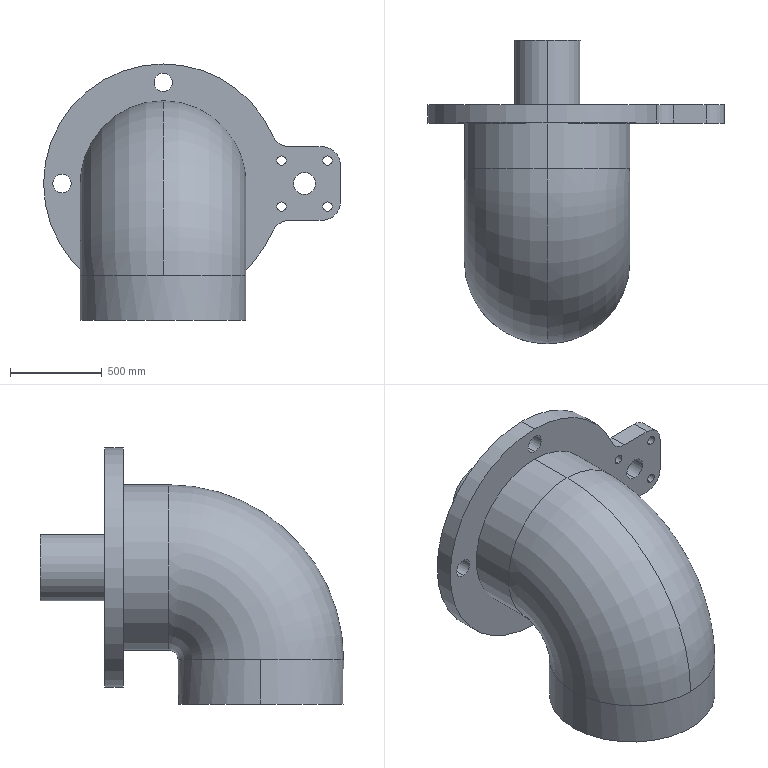Part | SolidWorks | features ICE 9, MoveFace 2, Extrusion 1, Fillet 1, MirrorPattern 1, Sweep 1 | 1 solid | 38 faces | box 1613 x 1648 x 1392 mm | volume 988148338 mm3 | cylinder 29 | plane 7 | torus 2 | commonest cylinder face diameters 50 x8 100 x6 200 x4 900 x4 1300 x3 120 x2
STEP:
#1=CARTESIAN_POINT('',(0.,-298.,-450.));
#2=VERTEX_POINT('',#1);
#3=CARTESIAN_POINT('',(0.,-298.,450.));
#4=VERTEX_POINT('',#3);
#5=CARTESIAN_POINT('',(0.,-298.,0.));
#6=DIRECTION('',(0.,-1.,0.));
#7=DIRECTION('',(0.,0.,-1.));
#8=AXIS2_PLACEMENT_3D('',#5,#6,#7);
#9=CIRCLE('',#8,450.);
#10=EDGE_CURVE('',#2,#4,#9,.T.);
#11=ORIENTED_EDGE('',*,*,#10,.T.);
#12=CARTESIAN_POINT('',(0.,-1248.,-500.));
#13=VERTEX_POINT('',#12);
#14=CARTESIAN_POINT('',(0.,-298.,-500.));
#15=DIRECTION('',(1.,0.,0.));
#16=DIRECTION('',(0.,0.,-1.));
#17=AXIS2_PLACEMENT_3D('',#14,#15,#16);
#18=CIRCLE('',#17,950.);
#19=EDGE_CURVE('',#4,#13,#18,.T.);
#20=ORIENTED_EDGE('',*,*,#19,.T.);
#21=CARTESIAN_POINT('',(450.,-798.,-500.));
#22=VERTEX_POINT('',#21);
#23=CARTESIAN_POINT('',(0.,-798.,-500.));
#24=DIRECTION('',(0.,0.,-1.));
#25=DIRECTION('',(0.,1.,0.));
#26=AXIS2_PLACEMENT_3D('',#23,#24,#25);
#27=CIRCLE('',#26,450.);
#28=EDGE_CURVE('',#22,#13,#27,.T.);
#29=ORIENTED_EDGE('',*,*,#28,.F.);
#30=CARTESIAN_POINT('',(0.,-348.,-500.));
#31=VERTEX_POINT('',#30);
#32=CARTESIAN_POINT('',(0.,-798.,-500.));
#33=DIRECTION('',(0.,0.,-1.));
#34=DIRECTION('',(0.,1.,0.));
#35=AXIS2_PLACEMENT_3D('',#32,#33,#34);
#36=CIRCLE('',#35,450.);
#37=EDGE_CURVE('',#31,#22,#36,.T.);
#38=ORIENTED_EDGE('',*,*,#37,.F.);
#39=CARTESIAN_POINT('',(0.,-298.,-500.));
#40=DIRECTION('',(1.,0.,0.));
#41=DIRECTION('',(0.,0.,-1.));
#42=AXIS2_PLACEMENT_3D('',#39,#40,#41);
#43=CIRCLE('',#42,50.);
#44=EDGE_CURVE('',#2,#31,#43,.T.);
#45=ORIENTED_EDGE('',*,*,#44,.F.);
#46=EDGE_LOOP('',(#11,#20,#29,#38,#45));
#47=FACE_OUTER_BOUND('',#46,.T.);
#48=CARTESIAN_POINT('',(0.,-298.,-500.));
#49=DIRECTION('',(1.,0.,0.));
#50=DIRECTION('',(0.,0.,-1.));
#51=AXIS2_PLACEMENT_3D('',#48,#49,#50);
#52=TOROIDAL_SURFACE('',#51,500.,450.);
#53=ADVANCED_FACE('',(#47),#52,.T.);
#54=CARTESIAN_POINT('',(-450.,-798.,-500.));
#55=VERTEX_POINT('',#54);
#56=CARTESIAN_POINT('',(0.,-798.,-500.));
#57=DIRECTION('',(0.,0.,-1.));
#58=DIRECTION('',(0.,1.,0.));
#59=AXIS2_PLACEMENT_3D('',#56,#57,#58);
#60=CIRCLE('',#59,450.);
#61=EDGE_CURVE('',#55,#31,#60,.T.);
#62=ORIENTED_EDGE('',*,*,#61,.T.);
#63=ORIENTED_EDGE('',*,*,#37,.T.);
#64=CARTESIAN_POINT('',(450.,-798.,-742.));
#65=VERTEX_POINT('',#64);
#66=CARTESIAN_POINT('',(450.,-798.,-500.));
#67=DIRECTION('',(0.,0.,-1.));
#68=VECTOR('',#67,1000.);
#69=LINE('',#66,#68);
#70=EDGE_CURVE('',#22,#65,#69,.T.);
#71=ORIENTED_EDGE('',*,*,#70,.T.);
#72=CARTESIAN_POINT('',(-450.,-798.,-742.));
#73=VERTEX_POINT('',#72);
#74=CARTESIAN_POINT('',(0.,-798.,-742.));
#75=DIRECTION('',(0.,0.,-1.));
#76=DIRECTION('',(0.,1.,0.));
#77=AXIS2_PLACEMENT_3D('',#74,#75,#76);
#78=CIRCLE('',#77,450.);
#79=EDGE_CURVE('',#73,#65,#78,.T.);
#80=ORIENTED_EDGE('',*,*,#79,.F.);
#81=CARTESIAN_POINT('',(-450.,-798.,-500.));
#82=DIRECTION('',(0.,0.,-1.));
#83=VECTOR('',#82,1000.);
#84=LINE('',#81,#83);
#85=EDGE_CURVE('',#55,#73,#84,.T.);
#86=ORIENTED_EDGE('',*,*,#85,.F.);
#87=EDGE_LOOP('',(#62,#63,#71,#80,#86));
#88=FACE_OUTER_BOUND('',#87,.T.);
#89=CARTESIAN_POINT('',(0.,-798.,-500.));
#90=DIRECTION('',(0.,0.,-1.));
#91=DIRECTION('',(-1.,0.,0.));
#92=AXIS2_PLACEMENT_3D('',#89,#90,#91);
#93=CYLINDRICAL_SURFACE('',#92,450.);
#94=ADVANCED_FACE('',(#88),#93,.T.);
#95=CARTESIAN_POINT('',(768.466,-50.,60.));
#96=VERTEX_POINT('',#95);
#97=CARTESIAN_POINT('',(768.466,-50.,-60.));
#98=VERTEX_POINT('',#97);
#99=CARTESIAN_POINT('',(768.466,-50.,0.));
#100=DIRECTION('',(0.,-1.,0.));
#101=DIRECTION('',(0.,0.,1.));
#102=AXIS2_PLACEMENT_3D('',#99,#100,#101);
#103=CIRCLE('',#102,60.);
#104=EDGE_CURVE('',#96,#98,#103,.T.);
#105=ORIENTED_EDGE('',*,*,#104,.T.);
#106=CARTESIAN_POINT('',(768.466,50.,-60.));
#107=VERTEX_POINT('',#106);
#108=CARTESIAN_POINT('',(768.466,-1050.001,-60.));
#109=DIRECTION('',(0.,1.,0.));
#110=VECTOR('',#109,1000.);
#111=LINE('',#108,#110);
#112=EDGE_CURVE('',#98,#107,#111,.T.);
#113=ORIENTED_EDGE('',*,*,#112,.T.);
#114=CARTESIAN_POINT('',(768.466,50.,60.));
#115=VERTEX_POINT('',#114);
#116=CARTESIAN_POINT('',(768.466,50.,0.));
#117=DIRECTION('',(0.,1.,0.));
#118=DIRECTION('',(0.,0.,1.));
#119=AXIS2_PLACEMENT_3D('',#116,#117,#118);
#120=CIRCLE('',#119,60.);
#121=EDGE_CURVE('',#107,#115,#120,.T.);
#122=ORIENTED_EDGE('',*,*,#121,.T.);
#123=CARTESIAN_POINT('',(768.466,-1050.001,60.));
#124=DIRECTION('',(0.,1.,0.));
#125=VECTOR('',#124,1000.);
#126=LINE('',#123,#125);
#127=EDGE_CURVE('',#96,#115,#126,.T.);
#128=ORIENTED_EDGE('',*,*,#127,.F.);
#129=EDGE_LOOP('',(#105,#113,#122,#128));
#130=FACE_OUTER_BOUND('',#129,.T.);
#131=CARTESIAN_POINT('',(768.466,-1050.001,0.));
#132=DIRECTION('',(0.,1.,0.));
#133=DIRECTION('',(0.,0.,1.));
#134=AXIS2_PLACEMENT_3D('',#131,#132,#133);
#135=CYLINDRICAL_SURFACE('',#134,60.);
#136=ADVANCED_FACE('',(#130),#135,.F.);
#137=CARTESIAN_POINT('',(893.466,-50.,150.));
#138=VERTEX_POINT('',#137);
#139=CARTESIAN_POINT('',(893.466,-50.,100.));
#140=VERTEX_POINT('',#139);
#141=CARTESIAN_POINT('',(893.466,-50.,125.));
#142=DIRECTION('',(0.,-1.,0.));
#143=DIRECTION('',(0.,0.,1.));
#144=AXIS2_PLACEMENT_3D('',#141,#142,#143);
#145=CIRCLE('',#144,25.);
#146=EDGE_CURVE('',#138,#140,#145,.T.);
#147=ORIENTED_EDGE('',*,*,#146,.T.);
#148=CARTESIAN_POINT('',(893.466,50.,100.));
#149=VERTEX_POINT('',#148);
#150=CARTESIAN_POINT('',(893.466,-1050.001,100.));
#151=DIRECTION('',(0.,1.,0.));
#152=VECTOR('',#151,1000.);
#153=LINE('',#150,#152);
#154=EDGE_CURVE('',#140,#149,#153,.T.);
#155=ORIENTED_EDGE('',*,*,#154,.T.);
#156=CARTESIAN_POINT('',(893.466,50.,150.));
#157=VERTEX_POINT('',#156);
#158=CARTESIAN_POINT('',(893.466,50.,125.));
#159=DIRECTION('',(0.,1.,0.));
#160=DIRECTION('',(0.,0.,1.));
#161=AXIS2_PLACEMENT_3D('',#158,#159,#160);
#162=CIRCLE('',#161,25.);
#163=EDGE_CURVE('',#149,#157,#162,.T.);
#164=ORIENTED_EDGE('',*,*,#163,.T.);
#165=CARTESIAN_POINT('',(893.466,-1050.001,150.));
#166=DIRECTION('',(0.,1.,0.));
#167=VECTOR('',#166,1000.);
#168=LINE('',#165,#167);
#169=EDGE_CURVE('',#138,#157,#168,.T.);
#170=ORIENTED_EDGE('',*,*,#169,.F.);
#171=EDGE_LOOP('',(#147,#155,#164,#170));
#172=FACE_OUTER_BOUND('',#171,.T.);
#173=CARTESIAN_POINT('',(893.466,-1050.001,125.));
#174=DIRECTION('',(0.,1.,0.));
#175=DIRECTION('',(0.,0.,1.));
#176=AXIS2_PLACEMENT_3D('',#173,#174,#175);
#177=CYLINDRICAL_SURFACE('',#176,25.);
#178=ADVANCED_FACE('',(#172),#177,.F.);
#179=CARTESIAN_POINT('',(643.466,-50.,150.));
#180=VERTEX_POINT('',#179);
#181=CARTESIAN_POINT('',(643.466,-50.,100.));
#182=VERTEX_POINT('',#181);
#183=CARTESIAN_POINT('',(643.466,-50.,125.));
#184=DIRECTION('',(0.,-1.,0.));
#185=DIRECTION('',(0.,0.,1.));
#186=AXIS2_PLACEMENT_3D('',#183,#184,#185);
#187=CIRCLE('',#186,25.);
#188=EDGE_CURVE('',#180,#182,#187,.T.);
#189=ORIENTED_EDGE('',*,*,#188,.T.);
#190=CARTESIAN_POINT('',(643.466,50.,100.));
#191=VERTEX_POINT('',#190);
#192=CARTESIAN_POINT('',(643.466,-1050.001,100.));
#193=DIRECTION('',(0.,1.,0.));
#194=VECTOR('',#193,1000.);
#195=LINE('',#192,#194);
#196=EDGE_CURVE('',#182,#191,#195,.T.);
#197=ORIENTED_EDGE('',*,*,#196,.T.);
#198=CARTESIAN_POINT('',(643.466,50.,150.));
#199=VERTEX_POINT('',#198);
#200=CARTESIAN_POINT('',(643.466,50.,125.));
#201=DIRECTION('',(0.,1.,0.));
#202=DIRECTION('',(0.,0.,1.));
#203=AXIS2_PLACEMENT_3D('',#200,#201,#202);
#204=CIRCLE('',#203,25.);
#205=EDGE_CURVE('',#191,#199,#204,.T.);
#206=ORIENTED_EDGE('',*,*,#205,.T.);
#207=CARTESIAN_POINT('',(643.466,-1050.001,150.));
#208=DIRECTION('',(0.,1.,0.));
#209=VECTOR('',#208,1000.);
#210=LINE('',#207,#209);
#211=EDGE_CURVE('',#180,#199,#210,.T.);
#212=ORIENTED_EDGE('',*,*,#211,.F.);
#213=EDGE_LOOP('',(#189,#197,#206,#212));
#214=FACE_OUTER_BOUND('',#213,.T.);
#215=CARTESIAN_POINT('',(643.466,-1050.001,125.));
#216=DIRECTION('',(0.,1.,0.));
#217=DIRECTION('',(0.,0.,1.));
#218=AXIS2_PLACEMENT_3D('',#215,#216,#217);
#219=CYLINDRICAL_SURFACE('',#218,25.);
#220=ADVANCED_FACE('',(#214),#219,.F.);
#221=CARTESIAN_POINT('',(643.466,-50.,-100.));
#222=VERTEX_POINT('',#221);
#223=CARTESIAN_POINT('',(643.466,-50.,-150.));
#224=VERTEX_POINT('',#223);
#225=CARTESIAN_POINT('',(643.466,-50.,-125.));
#226=DIRECTION('',(0.,-1.,0.));
#227=DIRECTION('',(0.,0.,1.));
#228=AXIS2_PLACEMENT_3D('',#225,#226,#227);
#229=CIRCLE('',#228,25.);
#230=EDGE_CURVE('',#222,#224,#229,.T.);
#231=ORIENTED_EDGE('',*,*,#230,.T.);
#232=CARTESIAN_POINT('',(643.466,50.,-150.));
#233=VERTEX_POINT('',#232);
#234=CARTESIAN_POINT('',(643.466,-1050.001,-150.));
#235=DIRECTION('',(0.,1.,0.));
#236=VECTOR('',#235,1000.);
#237=LINE('',#234,#236);
#238=EDGE_CURVE('',#224,#233,#237,.T.);
#239=ORIENTED_EDGE('',*,*,#238,.T.);
#240=CARTESIAN_POINT('',(643.466,50.,-100.));
#241=VERTEX_POINT('',#240);
#242=CARTESIAN_POINT('',(643.466,50.,-125.));
#243=DIRECTION('',(0.,1.,0.));
#244=DIRECTION('',(0.,0.,1.));
#245=AXIS2_PLACEMENT_3D('',#242,#243,#244);
#246=CIRCLE('',#245,25.);
#247=EDGE_CURVE('',#233,#241,#246,.T.);
#248=ORIENTED_EDGE('',*,*,#247,.T.);
#249=CARTESIAN_POINT('',(643.466,-1050.001,-100.));
#250=DIRECTION('',(0.,1.,0.));
#251=VECTOR('',#250,1000.);
#252=LINE('',#249,#251);
#253=EDGE_CURVE('',#222,#241,#252,.T.);
#254=ORIENTED_EDGE('',*,*,#253,.F.);
#255=EDGE_LOOP('',(#231,#239,#248,#254));
#256=FACE_OUTER_BOUND('',#255,.T.);
#257=CARTESIAN_POINT('',(643.466,-1050.001,-125.));
#258=DIRECTION('',(0.,1.,0.));
#259=DIRECTION('',(0.,0.,1.));
#260=AXIS2_PLACEMENT_3D('',#257,#258,#259);
#261=CYLINDRICAL_SURFACE('',#260,25.);
#262=ADVANCED_FACE('',(#256),#261,.F.);
#263=CARTESIAN_POINT('',(893.466,-50.,-100.));
#264=VERTEX_POINT('',#263);
#265=CARTESIAN_POINT('',(893.466,-50.,-150.));
#266=VERTEX_POINT('',#265);
#267=CARTESIAN_POINT('',(893.466,-50.,-125.));
#268=DIRECTION('',(0.,-1.,0.));
#269=DIRECTION('',(0.,0.,1.));
#270=AXIS2_PLACEMENT_3D('',#267,#268,#269);
#271=CIRCLE('',#270,25.);
#272=EDGE_CURVE('',#264,#266,#271,.T.);
#273=ORIENTED_EDGE('',*,*,#272,.T.);
#274=CARTESIAN_POINT('',(893.466,50.,-150.));
#275=VERTEX_POINT('',#274);
#276=CARTESIAN_POINT('',(893.466,-1050.001,-150.));
#277=DIRECTION('',(0.,1.,0.));
#278=VECTOR('',#277,1000.);
#279=LINE('',#276,#278);
#280=EDGE_CURVE('',#266,#275,#279,.T.);
#281=ORIENTED_EDGE('',*,*,#280,.T.);
#282=CARTESIAN_POINT('',(893.466,50.,-100.));
#283=VERTEX_POINT('',#282);
#284=CARTESIAN_POINT('',(893.466,50.,-125.));
#285=DIRECTION('',(0.,1.,0.));
#286=DIRECTION('',(0.,0.,1.));
#287=AXIS2_PLACEMENT_3D('',#284,#285,#286);
#288=CIRCLE('',#287,25.);
#289=EDGE_CURVE('',#275,#283,#288,.T.);
#290=ORIENTED_EDGE('',*,*,#289,.T.);
#291=CARTESIAN_POINT('',(893.466,-1050.001,-100.));
#292=DIRECTION('',(0.,1.,0.));
#293=VECTOR('',#292,1000.);
#294=LINE('',#291,#293);
#295=EDGE_CURVE('',#264,#283,#294,.T.);
#296=ORIENTED_EDGE('',*,*,#295,.F.);
#297=EDGE_LOOP('',(#273,#281,#290,#296));
#298=FACE_OUTER_BOUND('',#297,.T.);
#299=CARTESIAN_POINT('',(893.466,-1050.001,-125.));
#300=DIRECTION('',(0.,1.,0.));
#301=DIRECTION('',(0.,0.,1.));
#302=AXIS2_PLACEMENT_3D('',#299,#300,#301);
#303=CYLINDRICAL_SURFACE('',#302,25.);
#304=ADVANCED_FACE('',(#298),#303,.F.);
#305=CARTESIAN_POINT('',(0.,400.,180.));
#306=VERTEX_POINT('',#305);
#307=CARTESIAN_POINT('',(0.,400.,-180.));
#308=VERTEX_POINT('',#307);
#309=CARTESIAN_POINT('',(0.,400.,0.));
#310=DIRECTION('',(0.,1.,0.));
#311=DIRECTION('',(0.,0.,1.));
#312=AXIS2_PLACEMENT_3D('',#309,#310,#311);
#313=CIRCLE('',#312,180.);
#314=EDGE_CURVE('',#306,#308,#313,.T.);
#315=ORIENTED_EDGE('',*,*,#314,.F.);
#316=CARTESIAN_POINT('',(0.,50.,180.));
#317=VERTEX_POINT('',#316);
#318=CARTESIAN_POINT('',(0.,1200.,180.));
#319=DIRECTION('',(0.,-1.,0.));
#320=VECTOR('',#319,1000.);
#321=LINE('',#318,#320);
#322=EDGE_CURVE('',#306,#317,#321,.T.);
#323=ORIENTED_EDGE('',*,*,#322,.T.);
#324=CARTESIAN_POINT('',(0.,50.,-180.));
#325=VERTEX_POINT('',#324);
#326=CARTESIAN_POINT('',(0.,50.,0.));
#327=DIRECTION('',(0.,1.,0.));
#328=DIRECTION('',(0.,0.,1.));
#329=AXIS2_PLACEMENT_3D('',#326,#327,#328);
#330=CIRCLE('',#329,180.);
#331=EDGE_CURVE('',#317,#325,#330,.T.);
#332=ORIENTED_EDGE('',*,*,#331,.T.);
#333=CARTESIAN_POINT('',(0.,1200.,-180.));
#334=DIRECTION('',(0.,-1.,0.));
#335=VECTOR('',#334,1000.);
#336=LINE('',#333,#335);
#337=EDGE_CURVE('',#308,#325,#336,.T.);
#338=ORIENTED_EDGE('',*,*,#337,.F.);
#339=EDGE_LOOP('',(#315,#323,#332,#338));
#340=FACE_OUTER_BOUND('',#339,.T.);
#341=CARTESIAN_POINT('',(0.,1200.,0.));
#342=DIRECTION('',(0.,-1.,0.));
#343=DIRECTION('',(0.,0.,-1.));
#344=AXIS2_PLACEMENT_3D('',#341,#342,#343);
#345=CYLINDRICAL_SURFACE('',#344,180.);
#346=ADVANCED_FACE('',(#340),#345,.T.);
#347=CARTESIAN_POINT('',(0.,-50.,600.));
#348=VERTEX_POINT('',#347);
#349=CARTESIAN_POINT('',(0.,-50.,500.));
#350=VERTEX_POINT('',#349);
#351=CARTESIAN_POINT('',(0.,-50.,550.));
#352=DIRECTION('',(0.,-1.,0.));
#353=DIRECTION('',(0.,0.,1.));
#354=AXIS2_PLACEMENT_3D('',#351,#352,#353);
#355=CIRCLE('',#354,50.);
#356=EDGE_CURVE('',#348,#350,#355,.T.);
#357=ORIENTED_EDGE('',*,*,#356,.T.);
#358=CARTESIAN_POINT('',(0.,50.,500.));
#359=VERTEX_POINT('',#358);
#360=CARTESIAN_POINT('',(0.,-1050.,500.));
#361=DIRECTION('',(0.,1.,0.));
#362=VECTOR('',#361,1000.);
#363=LINE('',#360,#362);
#364=EDGE_CURVE('',#350,#359,#363,.T.);
#365=ORIENTED_EDGE('',*,*,#364,.T.);
#366=CARTESIAN_POINT('',(0.,50.,600.));
#367=VERTEX_POINT('',#366);
#368=CARTESIAN_POINT('',(0.,50.,550.));
#369=DIRECTION('',(0.,-1.,0.));
#370=DIRECTION('',(0.,0.,-1.));
#371=AXIS2_PLACEMENT_3D('',#368,#369,#370);
#372=CIRCLE('',#371,50.);
#373=EDGE_CURVE('',#367,#359,#372,.T.);
#374=ORIENTED_EDGE('',*,*,#373,.F.);
#375=CARTESIAN_POINT('',(0.,-1050.,600.));
#376=DIRECTION('',(0.,1.,0.));
#377=VECTOR('',#376,1000.);
#378=LINE('',#375,#377);
#379=EDGE_CURVE('',#348,#367,#378,.T.);
#380=ORIENTED_EDGE('',*,*,#379,.F.);
#381=EDGE_LOOP('',(#357,#365,#374,#380));
#382=FACE_OUTER_BOUND('',#381,.T.);
#383=CARTESIAN_POINT('',(0.,-1050.,550.));
#384=DIRECTION('',(0.,1.,0.));
#385=DIRECTION('',(0.,0.,1.));
#386=AXIS2_PLACEMENT_3D('',#383,#384,#385);
#387=CYLINDRICAL_SURFACE('',#386,50.);
#388=ADVANCED_FACE('',(#382),#387,.F.);
#389=CARTESIAN_POINT('',(0.,-50.,-500.));
#390=VERTEX_POINT('',#389);
#391=CARTESIAN_POINT('',(0.,-50.,-600.));
#392=VERTEX_POINT('',#391);
#393=CARTESIAN_POINT('',(0.,-50.,-550.));
#394=DIRECTION('',(0.,-1.,0.));
#395=DIRECTION('',(0.,0.,1.));
#396=AXIS2_PLACEMENT_3D('',#393,#394,#395);
#397=CIRCLE('',#396,50.);
#398=EDGE_CURVE('',#390,#392,#397,.T.);
#399=ORIENTED_EDGE('',*,*,#398,.T.);
#400=CARTESIAN_POINT('',(0.,50.,-600.));
#401=VERTEX_POINT('',#400);
#402=CARTESIAN_POINT('',(0.,-1050.,-600.));
#403=DIRECTION('',(0.,1.,0.));
#404=VECTOR('',#403,1000.);
#405=LINE('',#402,#404);
#406=EDGE_CURVE('',#392,#401,#405,.T.);
#407=ORIENTED_EDGE('',*,*,#406,.T.);
#408=CARTESIAN_POINT('',(0.,50.,-500.));
#409=VERTEX_POINT('',#408);
#410=CARTESIAN_POINT('',(0.,50.,-550.));
#411=DIRECTION('',(0.,-1.,0.));
#412=DIRECTION('',(0.,0.,-1.));
#413=AXIS2_PLACEMENT_3D('',#410,#411,#412);
#414=CIRCLE('',#413,50.);
#415=EDGE_CURVE('',#409,#401,#414,.T.);
#416=ORIENTED_EDGE('',*,*,#415,.F.);
#417=CARTESIAN_POINT('',(0.,-1050.,-500.));
#418=DIRECTION('',(0.,1.,0.));
#419=VECTOR('',#418,1000.);
#420=LINE('',#417,#419);
#421=EDGE_CURVE('',#390,#409,#420,.T.);
#422=ORIENTED_EDGE('',*,*,#421,.F.);
#423=EDGE_LOOP('',(#399,#407,#416,#422));
#424=FACE_OUTER_BOUND('',#423,.T.);
#425=CARTESIAN_POINT('',(0.,-1050.,-550.));
#426=DIRECTION('',(0.,1.,0.));
#427=DIRECTION('',(0.,0.,1.));
#428=AXIS2_PLACEMENT_3D('',#425,#426,#427);
#429=CYLINDRICAL_SURFACE('',#428,50.);
#430=ADVANCED_FACE('',(#424),#429,.F.);
#431=CARTESIAN_POINT('',(-550.,-50.,50.));
#432=VERTEX_POINT('',#431);
#433=CARTESIAN_POINT('',(-550.,-50.,-50.));
#434=VERTEX_POINT('',#433);
#435=CARTESIAN_POINT('',(-550.,-50.,0.));
#436=DIRECTION('',(0.,-1.,0.));
#437=DIRECTION('',(0.,0.,1.));
#438=AXIS2_PLACEMENT_3D('',#435,#436,#437);
#439=CIRCLE('',#438,50.);
#440=EDGE_CURVE('',#432,#434,#439,.T.);
#441=ORIENTED_EDGE('',*,*,#440,.T.);
#442=CARTESIAN_POINT('',(-550.,50.,-50.));
#443=VERTEX_POINT('',#442);
#444=CARTESIAN_POINT('',(-550.,-1050.,-50.));
#445=DIRECTION('',(0.,1.,0.));
#446=VECTOR('',#445,1000.);
#447=LINE('',#444,#446);
#448=EDGE_CURVE('',#434,#443,#447,.T.);
#449=ORIENTED_EDGE('',*,*,#448,.T.);
#450=CARTESIAN_POINT('',(-550.,50.,50.));
#451=VERTEX_POINT('',#450);
#452=CARTESIAN_POINT('',(-550.,50.,0.));
#453=DIRECTION('',(0.,-1.,0.));
#454=DIRECTION('',(0.,0.,-1.));
#455=AXIS2_PLACEMENT_3D('',#452,#453,#454);
#456=CIRCLE('',#455,50.);
#457=EDGE_CURVE('',#451,#443,#456,.T.);
#458=ORIENTED_EDGE('',*,*,#457,.F.);
#459=CARTESIAN_POINT('',(-550.,-1050.,50.));
#460=DIRECTION('',(0.,1.,0.));
#461=VECTOR('',#460,1000.);
#462=LINE('',#459,#461);
#463=EDGE_CURVE('',#432,#451,#462,.T.);
#464=ORIENTED_EDGE('',*,*,#463,.F.);
#465=EDGE_LOOP('',(#441,#449,#458,#464));
#466=FACE_OUTER_BOUND('',#465,.T.);
#467=CARTESIAN_POINT('',(-550.,-1050.,0.));
#468=DIRECTION('',(0.,1.,0.));
#469=DIRECTION('',(0.,0.,1.));
#470=AXIS2_PLACEMENT_3D('',#467,#468,#469);
#471=CYLINDRICAL_SURFACE('',#470,50.);
#472=ADVANCED_FACE('',(#466),#471,.F.);
#473=CARTESIAN_POINT('',(595.735,50.,260.));
#474=VERTEX_POINT('',#473);
#475=CARTESIAN_POINT('',(0.,50.,650.));
#476=VERTEX_POINT('',#475);
#477=CARTESIAN_POINT('',(0.,50.,0.));
#478=DIRECTION('',(0.,-1.,0.));
#479=DIRECTION('',(0.,0.,-1.));
#480=AXIS2_PLACEMENT_3D('',#477,#478,#479);
#481=CIRCLE('',#480,650.);
#482=EDGE_CURVE('',#474,#476,#481,.T.);
#483=ORIENTED_EDGE('',*,*,#482,.T.);
#484=CARTESIAN_POINT('',(0.,-50.,650.));
#485=VERTEX_POINT('',#484);
#486=CARTESIAN_POINT('',(0.,850.,650.));
#487=DIRECTION('',(0.,-1.,0.));
#488=VECTOR('',#487,1000.);
#489=LINE('',#486,#488);
#490=EDGE_CURVE('',#476,#485,#489,.T.);
#491=ORIENTED_EDGE('',*,*,#490,.T.);
#492=CARTESIAN_POINT('',(595.735,-50.,260.));
#493=VERTEX_POINT('',#492);
#494=CARTESIAN_POINT('',(0.,-50.,0.));
#495=DIRECTION('',(0.,-1.,0.));
#496=DIRECTION('',(0.,0.,-1.));
#497=AXIS2_PLACEMENT_3D('',#494,#495,#496);
#498=CIRCLE('',#497,650.);
#499=EDGE_CURVE('',#493,#485,#498,.T.);
#500=ORIENTED_EDGE('',*,*,#499,.F.);
#501=CARTESIAN_POINT('',(595.735,850.,260.));
#502=DIRECTION('',(0.,1.,0.));
#503=VECTOR('',#502,1000.);
#504=LINE('',#501,#503);
#505=EDGE_CURVE('',#493,#474,#504,.T.);
#506=ORIENTED_EDGE('',*,*,#505,.T.);
#507=EDGE_LOOP('',(#483,#491,#500,#506));
#508=FACE_OUTER_BOUND('',#507,.T.);
#509=CARTESIAN_POINT('',(0.,850.,0.));
#510=DIRECTION('',(0.,-1.,0.));
#511=DIRECTION('',(0.,0.,-1.));
#512=AXIS2_PLACEMENT_3D('',#509,#510,#511);
#513=CYLINDRICAL_SURFACE('',#512,650.);
#514=ADVANCED_FACE('',(#508),#513,.T.);
#515=ORIENTED_EDGE('',*,*,#490,.F.);
#516=CARTESIAN_POINT('',(0.,50.,-650.));
#517=VERTEX_POINT('',#516);
#518=CARTESIAN_POINT('',(0.,50.,0.));
#519=DIRECTION('',(0.,-1.,0.));
#520=DIRECTION('',(0.,0.,-1.));
#521=AXIS2_PLACEMENT_3D('',#518,#519,#520);
#522=CIRCLE('',#521,650.);
#523=EDGE_CURVE('',#476,#517,#522,.T.);
#524=ORIENTED_EDGE('',*,*,#523,.T.);
#525=CARTESIAN_POINT('',(0.,-50.,-650.));
#526=VERTEX_POINT('',#525);
#527=CARTESIAN_POINT('',(0.,850.,-650.));
#528=DIRECTION('',(0.,-1.,0.));
#529=VECTOR('',#528,1000.);
#530=LINE('',#527,#529);
#531=EDGE_CURVE('',#517,#526,#530,.T.);
#532=ORIENTED_EDGE('',*,*,#531,.T.);
#533=CARTESIAN_POINT('',(0.,-50.,0.));
#534=DIRECTION('',(0.,-1.,0.));
#535=DIRECTION('',(0.,0.,-1.));
#536=AXIS2_PLACEMENT_3D('',#533,#534,#535);
#537=CIRCLE('',#536,650.);
#538=EDGE_CURVE('',#485,#526,#537,.T.);
#539=ORIENTED_EDGE('',*,*,#538,.F.);
#540=EDGE_LOOP('',(#515,#524,#532,#539));
#541=FACE_OUTER_BOUND('',#540,.T.);
#542=CARTESIAN_POINT('',(0.,850.,0.));
#543=DIRECTION('',(0.,-1.,0.));
#544=DIRECTION('',(0.,0.,-1.));
#545=AXIS2_PLACEMENT_3D('',#542,#543,#544);
#546=CYLINDRICAL_SURFACE('',#545,650.);
#547=ADVANCED_FACE('',(#541),#546,.T.);
#548=CARTESIAN_POINT('',(0.,-50.,450.));
#549=VERTEX_POINT('',#548);
#550=CARTESIAN_POINT('',(0.,-50.,-450.));
#551=VERTEX_POINT('',#550);
#552=CARTESIAN_POINT('',(0.,-50.,0.));
#553=DIRECTION('',(0.,1.,0.));
#554=DIRECTION('',(0.,0.,1.));
#555=AXIS2_PLACEMENT_3D('',#552,#553,#554);
#556=CIRCLE('',#555,450.);
#557=EDGE_CURVE('',#549,#551,#556,.T.);
#558=ORIENTED_EDGE('',*,*,#557,.F.);
#559=CARTESIAN_POINT('',(0.,750.,450.));
#560=DIRECTION('',(0.,-1.,0.));
#561=VECTOR('',#560,1000.);
#562=LINE('',#559,#561);
#563=EDGE_CURVE('',#549,#4,#562,.T.);
#564=ORIENTED_EDGE('',*,*,#563,.T.);
#565=ORIENTED_EDGE('',*,*,#10,.F.);
#566=CARTESIAN_POINT('',(0.,750.,-450.));
#567=DIRECTION('',(0.,-1.,0.));
#568=VECTOR('',#567,1000.);
#569=LINE('',#566,#568);
#570=EDGE_CURVE('',#551,#2,#569,.T.);
#571=ORIENTED_EDGE('',*,*,#570,.F.);
#572=EDGE_LOOP('',(#558,#564,#565,#571));
#573=FACE_OUTER_BOUND('',#572,.T.);
#574=CARTESIAN_POINT('',(0.,750.,0.));
#575=DIRECTION('',(0.,-1.,0.));
#576=DIRECTION('',(0.,0.,-1.));
#577=AXIS2_PLACEMENT_3D('',#574,#575,#576);
#578=CYLINDRICAL_SURFACE('',#577,450.);
#579=ADVANCED_FACE('',(#573),#578,.T.);
#580=ORIENTED_EDGE('',*,*,#563,.F.);
#581=CARTESIAN_POINT('',(0.,-50.,0.));
#582=DIRECTION('',(0.,1.,0.));
#583=DIRECTION('',(0.,0.,1.));
#584=AXIS2_PLACEMENT_3D('',#581,#582,#583);
#585=CIRCLE('',#584,450.);
#586=EDGE_CURVE('',#551,#549,#585,.T.);
#587=ORIENTED_EDGE('',*,*,#586,.F.);
#588=ORIENTED_EDGE('',*,*,#570,.T.);
#589=CARTESIAN_POINT('',(0.,-298.,0.));
#590=DIRECTION('',(0.,-1.,0.));
#591=DIRECTION('',(0.,0.,-1.));
#592=AXIS2_PLACEMENT_3D('',#589,#590,#591);
#593=CIRCLE('',#592,450.);
#594=EDGE_CURVE('',#4,#2,#593,.T.);
#595=ORIENTED_EDGE('',*,*,#594,.F.);
#596=EDGE_LOOP('',(#580,#587,#588,#595));
#597=FACE_OUTER_BOUND('',#596,.T.);
#598=CARTESIAN_POINT('',(0.,750.,0.));
#599=DIRECTION('',(0.,-1.,0.));
#600=DIRECTION('',(0.,0.,-1.));
#601=AXIS2_PLACEMENT_3D('',#598,#599,#600);
#602=CYLINDRICAL_SURFACE('',#601,450.);
#603=ADVANCED_FACE('',(#597),#602,.T.);
#604=ORIENTED_EDGE('',*,*,#531,.F.);
#605=CARTESIAN_POINT('',(595.735,50.,-260.));
#606=VERTEX_POINT('',#605);
#607=CARTESIAN_POINT('',(0.,50.,0.));
#608=DIRECTION('',(0.,-1.,0.));
#609=DIRECTION('',(0.,0.,-1.));
#610=AXIS2_PLACEMENT_3D('',#607,#608,#609);
#611=CIRCLE('',#610,650.);
#612=EDGE_CURVE('',#517,#606,#611,.T.);
#613=ORIENTED_EDGE('',*,*,#612,.T.);
#614=CARTESIAN_POINT('',(595.735,-50.,-260.));
#615=VERTEX_POINT('',#614);
#616=CARTESIAN_POINT('',(595.735,850.,-260.));
#617=DIRECTION('',(0.,-1.,0.));
#618=VECTOR('',#617,1000.);
#619=LINE('',#616,#618);
#620=EDGE_CURVE('',#606,#615,#619,.T.);
#621=ORIENTED_EDGE('',*,*,#620,.T.);
#622=CARTESIAN_POINT('',(0.,-50.,0.));
#623=DIRECTION('',(0.,-1.,0.));
#624=DIRECTION('',(0.,0.,-1.));
#625=AXIS2_PLACEMENT_3D('',#622,#623,#624);
#626=CIRCLE('',#625,650.);
#627=EDGE_CURVE('',#526,#615,#626,.T.);
#628=ORIENTED_EDGE('',*,*,#627,.F.);
#629=EDGE_LOOP('',(#604,#613,#621,#628));
#630=FACE_OUTER_BOUND('',#629,.T.);
#631=CARTESIAN_POINT('',(0.,850.,0.));
#632=DIRECTION('',(0.,-1.,0.));
#633=DIRECTION('',(0.,0.,-1.));
#634=AXIS2_PLACEMENT_3D('',#631,#632,#633);
#635=CYLINDRICAL_SURFACE('',#634,650.);
#636=ADVANCED_FACE('',(#630),#635,.T.);
#637=CARTESIAN_POINT('',(768.466,50.,0.));
#638=DIRECTION('',(0.,1.,0.));
#639=DIRECTION('',(0.,0.,1.));
#640=AXIS2_PLACEMENT_3D('',#637,#638,#639);
#641=CIRCLE('',#640,60.);
#642=EDGE_CURVE('',#115,#107,#641,.T.);
#643=ORIENTED_EDGE('',*,*,#642,.F.);
#644=ORIENTED_EDGE('',*,*,#121,.F.);
#645=EDGE_LOOP('',(#643,#644));
#646=FACE_BOUND('',#645,.T.);
#647=CARTESIAN_POINT('',(893.466,50.,125.));
#648=DIRECTION('',(0.,1.,0.));
#649=DIRECTION('',(0.,0.,1.));
#650=AXIS2_PLACEMENT_3D('',#647,#648,#649);
#651=CIRCLE('',#650,25.);
#652=EDGE_CURVE('',#157,#149,#651,.T.);
#653=ORIENTED_EDGE('',*,*,#652,.F.);
#654=ORIENTED_EDGE('',*,*,#163,.F.);
#655=EDGE_LOOP('',(#653,#654));
#656=FACE_BOUND('',#655,.T.);
#657=CARTESIAN_POINT('',(643.466,50.,125.));
#658=DIRECTION('',(0.,1.,0.));
#659=DIRECTION('',(0.,0.,1.));
#660=AXIS2_PLACEMENT_3D('',#657,#658,#659);
#661=CIRCLE('',#660,25.);
#662=EDGE_CURVE('',#199,#191,#661,.T.);
#663=ORIENTED_EDGE('',*,*,#662,.F.);
#664=ORIENTED_EDGE('',*,*,#205,.F.);
#665=EDGE_LOOP('',(#663,#664));
#666=FACE_BOUND('',#665,.T.);
#667=CARTESIAN_POINT('',(643.466,50.,-125.));
#668=DIRECTION('',(0.,1.,0.));
#669=DIRECTION('',(0.,0.,1.));
#670=AXIS2_PLACEMENT_3D('',#667,#668,#669);
#671=CIRCLE('',#670,25.);
#672=EDGE_CURVE('',#241,#233,#671,.T.);
#673=ORIENTED_EDGE('',*,*,#672,.F.);
#674=ORIENTED_EDGE('',*,*,#247,.F.);
#675=EDGE_LOOP('',(#673,#674));
#676=FACE_BOUND('',#675,.T.);
#677=CARTESIAN_POINT('',(893.466,50.,-125.));
#678=DIRECTION('',(0.,1.,0.));
#679=DIRECTION('',(0.,0.,1.));
#680=AXIS2_PLACEMENT_3D('',#677,#678,#679);
#681=CIRCLE('',#680,25.);
#682=EDGE_CURVE('',#283,#275,#681,.T.);
#683=ORIENTED_EDGE('',*,*,#682,.F.);
#684=ORIENTED_EDGE('',*,*,#289,.F.);
#685=EDGE_LOOP('',(#683,#684));
#686=FACE_BOUND('',#685,.T.);
#687=CARTESIAN_POINT('',(687.386,50.,200.));
#688=VERTEX_POINT('',#687);
#689=CARTESIAN_POINT('',(863.466,50.,200.));
#690=VERTEX_POINT('',#689);
#691=CARTESIAN_POINT('',(618.466,50.,200.));
#692=DIRECTION('',(1.,0.,0.));
#693=VECTOR('',#692,1000.);
#694=LINE('',#691,#693);
#695=EDGE_CURVE('',#688,#690,#694,.T.);
#696=ORIENTED_EDGE('',*,*,#695,.T.);
#697=CARTESIAN_POINT('',(963.466,50.,100.));
#698=VERTEX_POINT('',#697);
#699=CARTESIAN_POINT('',(863.466,50.,100.));
#700=DIRECTION('',(0.,1.,0.));
#701=DIRECTION('',(0.,0.,1.));
#702=AXIS2_PLACEMENT_3D('',#699,#700,#701);
#703=CIRCLE('',#702,100.);
#704=EDGE_CURVE('',#690,#698,#703,.T.);
#705=ORIENTED_EDGE('',*,*,#704,.T.);
#706=CARTESIAN_POINT('',(963.466,50.,-100.));
#707=VERTEX_POINT('',#706);
#708=CARTESIAN_POINT('',(963.466,50.,-200.));
#709=DIRECTION('',(0.,0.,-1.));
#710=VECTOR('',#709,1000.);
#711=LINE('',#708,#710);
#712=EDGE_CURVE('',#698,#707,#711,.T.);
#713=ORIENTED_EDGE('',*,*,#712,.T.);
#714=CARTESIAN_POINT('',(863.466,50.,-200.));
#715=VERTEX_POINT('',#714);
#716=CARTESIAN_POINT('',(863.466,50.,-100.));
#717=DIRECTION('',(0.,1.,0.));
#718=DIRECTION('',(0.,0.,1.));
#719=AXIS2_PLACEMENT_3D('',#716,#717,#718);
#720=CIRCLE('',#719,100.);
#721=EDGE_CURVE('',#707,#715,#720,.T.);
#722=ORIENTED_EDGE('',*,*,#721,.T.);
#723=CARTESIAN_POINT('',(687.386,50.,-200.));
#724=VERTEX_POINT('',#723);
#725=CARTESIAN_POINT('',(618.466,50.,-200.));
#726=DIRECTION('',(-1.,0.,0.));
#727=VECTOR('',#726,1000.);
#728=LINE('',#725,#727);
#729=EDGE_CURVE('',#715,#724,#728,.T.);
#730=ORIENTED_EDGE('',*,*,#729,.T.);
#731=CARTESIAN_POINT('',(687.386,50.,-300.));
#732=DIRECTION('',(0.,-1.,0.));
#733=DIRECTION('',(0.,0.,1.));
#734=AXIS2_PLACEMENT_3D('',#731,#732,#733);
#735=CIRCLE('',#734,100.);
#736=EDGE_CURVE('',#724,#606,#735,.T.);
#737=ORIENTED_EDGE('',*,*,#736,.T.);
#738=ORIENTED_EDGE('',*,*,#612,.F.);
#739=ORIENTED_EDGE('',*,*,#523,.F.);
#740=ORIENTED_EDGE('',*,*,#482,.F.);
#741=CARTESIAN_POINT('',(687.386,50.,300.));
#742=DIRECTION('',(0.,-1.,0.));
#743=DIRECTION('',(0.,0.,1.));
#744=AXIS2_PLACEMENT_3D('',#741,#742,#743);
#745=CIRCLE('',#744,100.);
#746=EDGE_CURVE('',#474,#688,#745,.T.);
#747=ORIENTED_EDGE('',*,*,#746,.T.);
#748=EDGE_LOOP('',(#696,#705,#713,#722,#730,#737,#738,#739,#740,#747));
#749=FACE_OUTER_BOUND('',#748,.T.);
#750=CARTESIAN_POINT('',(0.,50.,0.));
#751=DIRECTION('',(0.,1.,0.));
#752=DIRECTION('',(0.,0.,1.));
#753=AXIS2_PLACEMENT_3D('',#750,#751,#752);
#754=CIRCLE('',#753,180.);
#755=EDGE_CURVE('',#325,#317,#754,.T.);
#756=ORIENTED_EDGE('',*,*,#755,.F.);
#757=ORIENTED_EDGE('',*,*,#331,.F.);
#758=EDGE_LOOP('',(#756,#757));
#759=FACE_BOUND('',#758,.T.);
#760=ORIENTED_EDGE('',*,*,#373,.T.);
#761=CARTESIAN_POINT('',(0.,50.,550.));
#762=DIRECTION('',(0.,-1.,0.));
#763=DIRECTION('',(0.,0.,-1.));
#764=AXIS2_PLACEMENT_3D('',#761,#762,#763);
#765=CIRCLE('',#764,50.);
#766=EDGE_CURVE('',#359,#367,#765,.T.);
#767=ORIENTED_EDGE('',*,*,#766,.T.);
#768=EDGE_LOOP('',(#760,#767));
#769=FACE_BOUND('',#768,.T.);
#770=ORIENTED_EDGE('',*,*,#415,.T.);
#771=CARTESIAN_POINT('',(0.,50.,-550.));
#772=DIRECTION('',(0.,-1.,0.));
#773=DIRECTION('',(0.,0.,-1.));
#774=AXIS2_PLACEMENT_3D('',#771,#772,#773);
#775=CIRCLE('',#774,50.);
#776=EDGE_CURVE('',#401,#409,#775,.T.);
#777=ORIENTED_EDGE('',*,*,#776,.T.);
#778=EDGE_LOOP('',(#770,#777));
#779=FACE_BOUND('',#778,.T.);
#780=ORIENTED_EDGE('',*,*,#457,.T.);
#781=CARTESIAN_POINT('',(-550.,50.,0.));
#782=DIRECTION('',(0.,-1.,0.));
#783=DIRECTION('',(0.,0.,-1.));
#784=AXIS2_PLACEMENT_3D('',#781,#782,#783);
#785=CIRCLE('',#784,50.);
#786=EDGE_CURVE('',#443,#451,#785,.T.);
#787=ORIENTED_EDGE('',*,*,#786,.T.);
#788=EDGE_LOOP('',(#780,#787));
#789=FACE_BOUND('',#788,.T.);
#790=CARTESIAN_POINT('',(0.,50.,0.));
#791=DIRECTION('',(0.,1.,0.));
#792=DIRECTION('',(0.,0.,-1.));
#793=AXIS2_PLACEMENT_3D('',#790,#791,#792);
#794=PLANE('',#793);
#795=ADVANCED_FACE('',(#646,#656,#666,#676,#686,#749,#759,#769,#779,#789),#794,.T.);
#796=ORIENTED_EDGE('',*,*,#104,.F.);
#797=CARTESIAN_POINT('',(768.466,-50.,0.));
#798=DIRECTION('',(0.,-1.,0.));
#799=DIRECTION('',(0.,0.,1.));
#800=AXIS2_PLACEMENT_3D('',#797,#798,#799);
#801=CIRCLE('',#800,60.);
#802=EDGE_CURVE('',#98,#96,#801,.T.);
#803=ORIENTED_EDGE('',*,*,#802,.F.);
#804=EDGE_LOOP('',(#796,#803));
#805=FACE_BOUND('',#804,.T.);
#806=ORIENTED_EDGE('',*,*,#146,.F.);
#807=CARTESIAN_POINT('',(893.466,-50.,125.));
#808=DIRECTION('',(0.,-1.,0.));
#809=DIRECTION('',(0.,0.,1.));
#810=AXIS2_PLACEMENT_3D('',#807,#808,#809);
#811=CIRCLE('',#810,25.);
#812=EDGE_CURVE('',#140,#138,#811,.T.);
#813=ORIENTED_EDGE('',*,*,#812,.F.);
#814=EDGE_LOOP('',(#806,#813));
#815=FACE_BOUND('',#814,.T.);
#816=ORIENTED_EDGE('',*,*,#188,.F.);
#817=CARTESIAN_POINT('',(643.466,-50.,125.));
#818=DIRECTION('',(0.,-1.,0.));
#819=DIRECTION('',(0.,0.,1.));
#820=AXIS2_PLACEMENT_3D('',#817,#818,#819);
#821=CIRCLE('',#820,25.);
#822=EDGE_CURVE('',#182,#180,#821,.T.);
#823=ORIENTED_EDGE('',*,*,#822,.F.);
#824=EDGE_LOOP('',(#816,#823));
#825=FACE_BOUND('',#824,.T.);
#826=ORIENTED_EDGE('',*,*,#230,.F.);
#827=CARTESIAN_POINT('',(643.466,-50.,-125.));
#828=DIRECTION('',(0.,-1.,0.));
#829=DIRECTION('',(0.,0.,1.));
#830=AXIS2_PLACEMENT_3D('',#827,#828,#829);
#831=CIRCLE('',#830,25.);
#832=EDGE_CURVE('',#224,#222,#831,.T.);
#833=ORIENTED_EDGE('',*,*,#832,.F.);
#834=EDGE_LOOP('',(#826,#833));
#835=FACE_BOUND('',#834,.T.);
#836=ORIENTED_EDGE('',*,*,#272,.F.);
#837=CARTESIAN_POINT('',(893.466,-50.,-125.));
#838=DIRECTION('',(0.,-1.,0.));
#839=DIRECTION('',(0.,0.,1.));
#840=AXIS2_PLACEMENT_3D('',#837,#838,#839);
#841=CIRCLE('',#840,25.);
#842=EDGE_CURVE('',#266,#264,#841,.T.);
#843=ORIENTED_EDGE('',*,*,#842,.F.);
#844=EDGE_LOOP('',(#836,#843));
#845=FACE_BOUND('',#844,.T.);
#846=ORIENTED_EDGE('',*,*,#356,.F.);
#847=CARTESIAN_POINT('',(0.,-50.,550.));
#848=DIRECTION('',(0.,-1.,0.));
#849=DIRECTION('',(0.,0.,1.));
#850=AXIS2_PLACEMENT_3D('',#847,#848,#849);
#851=CIRCLE('',#850,50.);
#852=EDGE_CURVE('',#350,#348,#851,.T.);
#853=ORIENTED_EDGE('',*,*,#852,.F.);
#854=EDGE_LOOP('',(#846,#853));
#855=FACE_BOUND('',#854,.T.);
#856=ORIENTED_EDGE('',*,*,#398,.F.);
#857=CARTESIAN_POINT('',(0.,-50.,-550.));
#858=DIRECTION('',(0.,-1.,0.));
#859=DIRECTION('',(0.,0.,1.));
#860=AXIS2_PLACEMENT_3D('',#857,#858,#859);
#861=CIRCLE('',#860,50.);
#862=EDGE_CURVE('',#392,#390,#861,.T.);
#863=ORIENTED_EDGE('',*,*,#862,.F.);
#864=EDGE_LOOP('',(#856,#863));
#865=FACE_BOUND('',#864,.T.);
#866=ORIENTED_EDGE('',*,*,#440,.F.);
#867=CARTESIAN_POINT('',(-550.,-50.,0.));
#868=DIRECTION('',(0.,-1.,0.));
#869=DIRECTION('',(0.,0.,1.));
#870=AXIS2_PLACEMENT_3D('',#867,#868,#869);
#871=CIRCLE('',#870,50.);
#872=EDGE_CURVE('',#434,#432,#871,.T.);
#873=ORIENTED_EDGE('',*,*,#872,.F.);
#874=EDGE_LOOP('',(#866,#873));
#875=FACE_BOUND('',#874,.T.);
#876=ORIENTED_EDGE('',*,*,#586,.T.);
#877=ORIENTED_EDGE('',*,*,#557,.T.);
#878=EDGE_LOOP('',(#876,#877));
#879=FACE_BOUND('',#878,.T.);
#880=CARTESIAN_POINT('',(963.466,-50.,-100.));
#881=VERTEX_POINT('',#880);
#882=CARTESIAN_POINT('',(963.466,-50.,100.));
#883=VERTEX_POINT('',#882);
#884=CARTESIAN_POINT('',(963.466,-50.,-200.));
#885=DIRECTION('',(0.,0.,1.));
#886=VECTOR('',#885,1000.);
#887=LINE('',#884,#886);
#888=EDGE_CURVE('',#881,#883,#887,.T.);
#889=ORIENTED_EDGE('',*,*,#888,.T.);
#890=CARTESIAN_POINT('',(863.466,-50.,200.));
#891=VERTEX_POINT('',#890);
#892=CARTESIAN_POINT('',(863.466,-50.,100.));
#893=DIRECTION('',(0.,-1.,0.));
#894=DIRECTION('',(0.,0.,1.));
#895=AXIS2_PLACEMENT_3D('',#892,#893,#894);
#896=CIRCLE('',#895,100.);
#897=EDGE_CURVE('',#883,#891,#896,.T.);
#898=ORIENTED_EDGE('',*,*,#897,.T.);
#899=CARTESIAN_POINT('',(687.386,-50.,200.));
#900=VERTEX_POINT('',#899);
#901=CARTESIAN_POINT('',(618.466,-50.,200.));
#902=DIRECTION('',(-1.,0.,0.));
#903=VECTOR('',#902,1000.);
#904=LINE('',#901,#903);
#905=EDGE_CURVE('',#891,#900,#904,.T.);
#906=ORIENTED_EDGE('',*,*,#905,.T.);
#907=CARTESIAN_POINT('',(687.386,-50.,300.));
#908=DIRECTION('',(0.,1.,0.));
#909=DIRECTION('',(0.,0.,1.));
#910=AXIS2_PLACEMENT_3D('',#907,#908,#909);
#911=CIRCLE('',#910,100.);
#912=EDGE_CURVE('',#900,#493,#911,.T.);
#913=ORIENTED_EDGE('',*,*,#912,.T.);
#914=ORIENTED_EDGE('',*,*,#499,.T.);
#915=ORIENTED_EDGE('',*,*,#538,.T.);
#916=ORIENTED_EDGE('',*,*,#627,.T.);
#917=CARTESIAN_POINT('',(687.386,-50.,-200.));
#918=VERTEX_POINT('',#917);
#919=CARTESIAN_POINT('',(687.386,-50.,-300.));
#920=DIRECTION('',(0.,1.,0.));
#921=DIRECTION('',(0.,0.,1.));
#922=AXIS2_PLACEMENT_3D('',#919,#920,#921);
#923=CIRCLE('',#922,100.);
#924=EDGE_CURVE('',#615,#918,#923,.T.);
#925=ORIENTED_EDGE('',*,*,#924,.T.);
#926=CARTESIAN_POINT('',(863.466,-50.,-200.));
#927=VERTEX_POINT('',#926);
#928=CARTESIAN_POINT('',(618.466,-50.,-200.));
#929=DIRECTION('',(1.,0.,0.));
#930=VECTOR('',#929,1000.);
#931=LINE('',#928,#930);
#932=EDGE_CURVE('',#918,#927,#931,.T.);
#933=ORIENTED_EDGE('',*,*,#932,.T.);
#934=CARTESIAN_POINT('',(863.466,-50.,-100.));
#935=DIRECTION('',(0.,-1.,0.));
#936=DIRECTION('',(0.,0.,1.));
#937=AXIS2_PLACEMENT_3D('',#934,#935,#936);
#938=CIRCLE('',#937,100.);
#939=EDGE_CURVE('',#927,#881,#938,.T.);
#940=ORIENTED_EDGE('',*,*,#939,.T.);
#941=EDGE_LOOP('',(#889,#898,#906,#913,#914,#915,#916,#925,#933,#940));
#942=FACE_OUTER_BOUND('',#941,.T.);
#943=CARTESIAN_POINT('',(0.,-50.,0.));
#944=DIRECTION('',(0.,1.,0.));
#945=DIRECTION('',(0.,0.,-1.));
#946=AXIS2_PLACEMENT_3D('',#943,#944,#945);
#947=PLANE('',#946);
#948=ADVANCED_FACE('',(#805,#815,#825,#835,#845,#855,#865,#875,#879,#942),#947,.F.);
#949=ORIENTED_EDGE('',*,*,#448,.F.);
#950=ORIENTED_EDGE('',*,*,#872,.T.);
#951=ORIENTED_EDGE('',*,*,#463,.T.);
#952=ORIENTED_EDGE('',*,*,#786,.F.);
#953=EDGE_LOOP('',(#949,#950,#951,#952));
#954=FACE_OUTER_BOUND('',#953,.T.);
#955=CARTESIAN_POINT('',(-550.,-1050.,0.));
#956=DIRECTION('',(0.,1.,0.));
#957=DIRECTION('',(0.,0.,1.));
#958=AXIS2_PLACEMENT_3D('',#955,#956,#957);
#959=CYLINDRICAL_SURFACE('',#958,50.);
#960=ADVANCED_FACE('',(#954),#959,.F.);
#961=ORIENTED_EDGE('',*,*,#406,.F.);
#962=ORIENTED_EDGE('',*,*,#862,.T.);
#963=ORIENTED_EDGE('',*,*,#421,.T.);
#964=ORIENTED_EDGE('',*,*,#776,.F.);
#965=EDGE_LOOP('',(#961,#962,#963,#964));
#966=FACE_OUTER_BOUND('',#965,.T.);
#967=CARTESIAN_POINT('',(0.,-1050.,-550.));
#968=DIRECTION('',(0.,1.,0.));
#969=DIRECTION('',(0.,0.,1.));
#970=AXIS2_PLACEMENT_3D('',#967,#968,#969);
#971=CYLINDRICAL_SURFACE('',#970,50.);
#972=ADVANCED_FACE('',(#966),#971,.F.);
#973=ORIENTED_EDGE('',*,*,#364,.F.);
#974=ORIENTED_EDGE('',*,*,#852,.T.);
#975=ORIENTED_EDGE('',*,*,#379,.T.);
#976=ORIENTED_EDGE('',*,*,#766,.F.);
#977=EDGE_LOOP('',(#973,#974,#975,#976));
#978=FACE_OUTER_BOUND('',#977,.T.);
#979=CARTESIAN_POINT('',(0.,-1050.,550.));
#980=DIRECTION('',(0.,1.,0.));
#981=DIRECTION('',(0.,0.,1.));
#982=AXIS2_PLACEMENT_3D('',#979,#980,#981);
#983=CYLINDRICAL_SURFACE('',#982,50.);
#984=ADVANCED_FACE('',(#978),#983,.F.);
#985=ORIENTED_EDGE('',*,*,#322,.F.);
#986=CARTESIAN_POINT('',(0.,400.,0.));
#987=DIRECTION('',(0.,1.,0.));
#988=DIRECTION('',(0.,0.,1.));
#989=AXIS2_PLACEMENT_3D('',#986,#987,#988);
#990=CIRCLE('',#989,180.);
#991=EDGE_CURVE('',#308,#306,#990,.T.);
#992=ORIENTED_EDGE('',*,*,#991,.F.);
#993=ORIENTED_EDGE('',*,*,#337,.T.);
#994=ORIENTED_EDGE('',*,*,#755,.T.);
#995=EDGE_LOOP('',(#985,#992,#993,#994));
#996=FACE_OUTER_BOUND('',#995,.T.);
#997=CARTESIAN_POINT('',(0.,1200.,0.));
#998=DIRECTION('',(0.,-1.,0.));
#999=DIRECTION('',(0.,0.,-1.));
#1000=AXIS2_PLACEMENT_3D('',#997,#998,#999);
#1001=CYLINDRICAL_SURFACE('',#1000,180.);
#1002=ADVANCED_FACE('',(#996),#1001,.T.);
#1003=ORIENTED_EDGE('',*,*,#991,.T.);
#1004=ORIENTED_EDGE('',*,*,#314,.T.);
#1005=EDGE_LOOP('',(#1003,#1004));
#1006=FACE_OUTER_BOUND('',#1005,.T.);
#1007=CARTESIAN_POINT('',(0.,400.,0.));
#1008=DIRECTION('',(0.,1.,0.));
#1009=DIRECTION('',(0.,0.,1.));
#1010=AXIS2_PLACEMENT_3D('',#1007,#1008,#1009);
#1011=PLANE('',#1010);
#1012=ADVANCED_FACE('',(#1006),#1011,.T.);
#1013=ORIENTED_EDGE('',*,*,#932,.F.);
#1014=CARTESIAN_POINT('',(687.386,850.,-200.));
#1015=DIRECTION('',(0.,1.,0.));
#1016=VECTOR('',#1015,1000.);
#1017=LINE('',#1014,#1016);
#1018=EDGE_CURVE('',#918,#724,#1017,.T.);
#1019=ORIENTED_EDGE('',*,*,#1018,.T.);
#1020=ORIENTED_EDGE('',*,*,#729,.F.);
#1021=CARTESIAN_POINT('',(863.466,221.772,-200.));
#1022=DIRECTION('',(0.,-1.,0.));
#1023=VECTOR('',#1022,1000.);
#1024=LINE('',#1021,#1023);
#1025=EDGE_CURVE('',#715,#927,#1024,.T.);
#1026=ORIENTED_EDGE('',*,*,#1025,.T.);
#1027=EDGE_LOOP('',(#1013,#1019,#1020,#1026));
#1028=FACE_OUTER_BOUND('',#1027,.T.);
#1029=CARTESIAN_POINT('',(618.466,221.772,-200.));
#1030=DIRECTION('',(0.,0.,-1.));
#1031=DIRECTION('',(-1.,0.,0.));
#1032=AXIS2_PLACEMENT_3D('',#1029,#1030,#1031);
#1033=PLANE('',#1032);
#1034=ADVANCED_FACE('',(#1028),#1033,.T.);
#1035=ORIENTED_EDGE('',*,*,#712,.F.);
#1036=CARTESIAN_POINT('',(963.466,221.772,100.));
#1037=DIRECTION('',(0.,-1.,0.));
#1038=VECTOR('',#1037,1000.);
#1039=LINE('',#1036,#1038);
#1040=EDGE_CURVE('',#698,#883,#1039,.T.);
#1041=ORIENTED_EDGE('',*,*,#1040,.T.);
#1042=ORIENTED_EDGE('',*,*,#888,.F.);
#1043=CARTESIAN_POINT('',(963.466,221.772,-100.));
#1044=DIRECTION('',(0.,1.,0.));
#1045=VECTOR('',#1044,1000.);
#1046=LINE('',#1043,#1045);
#1047=EDGE_CURVE('',#881,#707,#1046,.T.);
#1048=ORIENTED_EDGE('',*,*,#1047,.T.);
#1049=EDGE_LOOP('',(#1035,#1041,#1042,#1048));
#1050=FACE_OUTER_BOUND('',#1049,.T.);
#1051=CARTESIAN_POINT('',(963.466,221.772,-200.));
#1052=DIRECTION('',(1.,0.,0.));
#1053=DIRECTION('',(0.,0.,-1.));
#1054=AXIS2_PLACEMENT_3D('',#1051,#1052,#1053);
#1055=PLANE('',#1054);
#1056=ADVANCED_FACE('',(#1050),#1055,.T.);
#1057=ORIENTED_EDGE('',*,*,#695,.F.);
#1058=CARTESIAN_POINT('',(687.386,750.,200.));
#1059=DIRECTION('',(0.,-1.,0.));
#1060=VECTOR('',#1059,1000.);
#1061=LINE('',#1058,#1060);
#1062=EDGE_CURVE('',#688,#900,#1061,.T.);
#1063=ORIENTED_EDGE('',*,*,#1062,.T.);
#1064=ORIENTED_EDGE('',*,*,#905,.F.);
#1065=CARTESIAN_POINT('',(863.466,221.772,200.));
#1066=DIRECTION('',(0.,1.,0.));
#1067=VECTOR('',#1066,1000.);
#1068=LINE('',#1065,#1067);
#1069=EDGE_CURVE('',#891,#690,#1068,.T.);
#1070=ORIENTED_EDGE('',*,*,#1069,.T.);
#1071=EDGE_LOOP('',(#1057,#1063,#1064,#1070));
#1072=FACE_OUTER_BOUND('',#1071,.T.);
#1073=CARTESIAN_POINT('',(618.466,221.772,200.));
#1074=DIRECTION('',(0.,0.,1.));
#1075=DIRECTION('',(1.,0.,0.));
#1076=AXIS2_PLACEMENT_3D('',#1073,#1074,#1075);
#1077=PLANE('',#1076);
#1078=ADVANCED_FACE('',(#1072),#1077,.T.);
#1079=ORIENTED_EDGE('',*,*,#280,.F.);
#1080=ORIENTED_EDGE('',*,*,#842,.T.);
#1081=ORIENTED_EDGE('',*,*,#295,.T.);
#1082=ORIENTED_EDGE('',*,*,#682,.T.);
#1083=EDGE_LOOP('',(#1079,#1080,#1081,#1082));
#1084=FACE_OUTER_BOUND('',#1083,.T.);
#1085=CARTESIAN_POINT('',(893.466,-1050.001,-125.));
#1086=DIRECTION('',(0.,1.,0.));
#1087=DIRECTION('',(0.,0.,1.));
#1088=AXIS2_PLACEMENT_3D('',#1085,#1086,#1087);
#1089=CYLINDRICAL_SURFACE('',#1088,25.);
#1090=ADVANCED_FACE('',(#1084),#1089,.F.);
#1091=ORIENTED_EDGE('',*,*,#238,.F.);
#1092=ORIENTED_EDGE('',*,*,#832,.T.);
#1093=ORIENTED_EDGE('',*,*,#253,.T.);
#1094=ORIENTED_EDGE('',*,*,#672,.T.);
#1095=EDGE_LOOP('',(#1091,#1092,#1093,#1094));
#1096=FACE_OUTER_BOUND('',#1095,.T.);
#1097=CARTESIAN_POINT('',(643.466,-1050.001,-125.));
#1098=DIRECTION('',(0.,1.,0.));
#1099=DIRECTION('',(0.,0.,1.));
#1100=AXIS2_PLACEMENT_3D('',#1097,#1098,#1099);
#1101=CYLINDRICAL_SURFACE('',#1100,25.);
#1102=ADVANCED_FACE('',(#1096),#1101,.F.);
#1103=ORIENTED_EDGE('',*,*,#196,.F.);
#1104=ORIENTED_EDGE('',*,*,#822,.T.);
#1105=ORIENTED_EDGE('',*,*,#211,.T.);
#1106=ORIENTED_EDGE('',*,*,#662,.T.);
#1107=EDGE_LOOP('',(#1103,#1104,#1105,#1106));
#1108=FACE_OUTER_BOUND('',#1107,.T.);
#1109=CARTESIAN_POINT('',(643.466,-1050.001,125.));
#1110=DIRECTION('',(0.,1.,0.));
#1111=DIRECTION('',(0.,0.,1.));
#1112=AXIS2_PLACEMENT_3D('',#1109,#1110,#1111);
#1113=CYLINDRICAL_SURFACE('',#1112,25.);
#1114=ADVANCED_FACE('',(#1108),#1113,.F.);
#1115=ORIENTED_EDGE('',*,*,#154,.F.);
#1116=ORIENTED_EDGE('',*,*,#812,.T.);
#1117=ORIENTED_EDGE('',*,*,#169,.T.);
#1118=ORIENTED_EDGE('',*,*,#652,.T.);
#1119=EDGE_LOOP('',(#1115,#1116,#1117,#1118));
#1120=FACE_OUTER_BOUND('',#1119,.T.);
#1121=CARTESIAN_POINT('',(893.466,-1050.001,125.));
#1122=DIRECTION('',(0.,1.,0.));
#1123=DIRECTION('',(0.,0.,1.));
#1124=AXIS2_PLACEMENT_3D('',#1121,#1122,#1123);
#1125=CYLINDRICAL_SURFACE('',#1124,25.);
#1126=ADVANCED_FACE('',(#1120),#1125,.F.);
#1127=ORIENTED_EDGE('',*,*,#112,.F.);
#1128=ORIENTED_EDGE('',*,*,#802,.T.);
#1129=ORIENTED_EDGE('',*,*,#127,.T.);
#1130=ORIENTED_EDGE('',*,*,#642,.T.);
#1131=EDGE_LOOP('',(#1127,#1128,#1129,#1130));
#1132=FACE_OUTER_BOUND('',#1131,.T.);
#1133=CARTESIAN_POINT('',(768.466,-1050.001,0.));
#1134=DIRECTION('',(0.,1.,0.));
#1135=DIRECTION('',(0.,0.,1.));
#1136=AXIS2_PLACEMENT_3D('',#1133,#1134,#1135);
#1137=CYLINDRICAL_SURFACE('',#1136,60.);
#1138=ADVANCED_FACE('',(#1132),#1137,.F.);
#1139=ORIENTED_EDGE('',*,*,#924,.F.);
#1140=ORIENTED_EDGE('',*,*,#620,.F.);
#1141=ORIENTED_EDGE('',*,*,#736,.F.);
#1142=ORIENTED_EDGE('',*,*,#1018,.F.);
#1143=EDGE_LOOP('',(#1139,#1140,#1141,#1142));
#1144=FACE_OUTER_BOUND('',#1143,.T.);
#1145=CARTESIAN_POINT('',(687.386,850.,-300.));
#1146=DIRECTION('',(0.,-1.,0.));
#1147=DIRECTION('',(0.,0.,-1.));
#1148=AXIS2_PLACEMENT_3D('',#1145,#1146,#1147);
#1149=CYLINDRICAL_SURFACE('',#1148,100.);
#1150=ADVANCED_FACE('',(#1144),#1149,.F.);
#1151=ORIENTED_EDGE('',*,*,#912,.F.);
#1152=ORIENTED_EDGE('',*,*,#1062,.F.);
#1153=ORIENTED_EDGE('',*,*,#746,.F.);
#1154=ORIENTED_EDGE('',*,*,#505,.F.);
#1155=EDGE_LOOP('',(#1151,#1152,#1153,#1154));
#1156=FACE_OUTER_BOUND('',#1155,.T.);
#1157=CARTESIAN_POINT('',(687.386,850.,300.));
#1158=DIRECTION('',(0.,-1.,0.));
#1159=DIRECTION('',(0.,0.,-1.));
#1160=AXIS2_PLACEMENT_3D('',#1157,#1158,#1159);
#1161=CYLINDRICAL_SURFACE('',#1160,100.);
#1162=ADVANCED_FACE('',(#1156),#1161,.F.);
#1163=ORIENTED_EDGE('',*,*,#897,.F.);
#1164=ORIENTED_EDGE('',*,*,#1040,.F.);
#1165=ORIENTED_EDGE('',*,*,#704,.F.);
#1166=ORIENTED_EDGE('',*,*,#1069,.F.);
#1167=EDGE_LOOP('',(#1163,#1164,#1165,#1166));
#1168=FACE_OUTER_BOUND('',#1167,.T.);
#1169=CARTESIAN_POINT('',(863.466,221.772,100.));
#1170=DIRECTION('',(0.,1.,0.));
#1171=DIRECTION('',(0.,0.,1.));
#1172=AXIS2_PLACEMENT_3D('',#1169,#1170,#1171);
#1173=CYLINDRICAL_SURFACE('',#1172,100.);
#1174=ADVANCED_FACE('',(#1168),#1173,.T.);
#1175=ORIENTED_EDGE('',*,*,#939,.F.);
#1176=ORIENTED_EDGE('',*,*,#1025,.F.);
#1177=ORIENTED_EDGE('',*,*,#721,.F.);
#1178=ORIENTED_EDGE('',*,*,#1047,.F.);
#1179=EDGE_LOOP('',(#1175,#1176,#1177,#1178));
#1180=FACE_OUTER_BOUND('',#1179,.T.);
#1181=CARTESIAN_POINT('',(863.466,221.772,-100.));
#1182=DIRECTION('',(0.,1.,0.));
#1183=DIRECTION('',(0.,0.,1.));
#1184=AXIS2_PLACEMENT_3D('',#1181,#1182,#1183);
#1185=CYLINDRICAL_SURFACE('',#1184,100.);
#1186=ADVANCED_FACE('',(#1180),#1185,.T.);
#1187=ORIENTED_EDGE('',*,*,#70,.F.);
#1188=ORIENTED_EDGE('',*,*,#28,.T.);
#1189=CARTESIAN_POINT('',(0.,-798.,-500.));
#1190=DIRECTION('',(0.,0.,-1.));
#1191=DIRECTION('',(0.,1.,0.));
#1192=AXIS2_PLACEMENT_3D('',#1189,#1190,#1191);
#1193=CIRCLE('',#1192,450.);
#1194=EDGE_CURVE('',#13,#55,#1193,.T.);
#1195=ORIENTED_EDGE('',*,*,#1194,.T.);
#1196=ORIENTED_EDGE('',*,*,#85,.T.);
#1197=CARTESIAN_POINT('',(0.,-798.,-742.));
#1198=DIRECTION('',(0.,0.,-1.));
#1199=DIRECTION('',(0.,1.,0.));
#1200=AXIS2_PLACEMENT_3D('',#1197,#1198,#1199);
#1201=CIRCLE('',#1200,450.);
#1202=EDGE_CURVE('',#65,#73,#1201,.T.);
#1203=ORIENTED_EDGE('',*,*,#1202,.F.);
#1204=EDGE_LOOP('',(#1187,#1188,#1195,#1196,#1203));
#1205=FACE_OUTER_BOUND('',#1204,.T.);
#1206=CARTESIAN_POINT('',(0.,-798.,-500.));
#1207=DIRECTION('',(0.,0.,-1.));
#1208=DIRECTION('',(-1.,0.,0.));
#1209=AXIS2_PLACEMENT_3D('',#1206,#1207,#1208);
#1210=CYLINDRICAL_SURFACE('',#1209,450.);
#1211=ADVANCED_FACE('',(#1205),#1210,.T.);
#1212=ORIENTED_EDGE('',*,*,#19,.F.);
#1213=ORIENTED_EDGE('',*,*,#594,.T.);
#1214=ORIENTED_EDGE('',*,*,#44,.T.);
#1215=ORIENTED_EDGE('',*,*,#61,.F.);
#1216=ORIENTED_EDGE('',*,*,#1194,.F.);
#1217=EDGE_LOOP('',(#1212,#1213,#1214,#1215,#1216));
#1218=FACE_OUTER_BOUND('',#1217,.T.);
#1219=CARTESIAN_POINT('',(0.,-298.,-500.));
#1220=DIRECTION('',(1.,0.,0.));
#1221=DIRECTION('',(0.,0.,-1.));
#1222=AXIS2_PLACEMENT_3D('',#1219,#1220,#1221);
#1223=TOROIDAL_SURFACE('',#1222,500.,450.);
#1224=ADVANCED_FACE('',(#1218),#1223,.T.);
#1225=ORIENTED_EDGE('',*,*,#79,.T.);
#1226=ORIENTED_EDGE('',*,*,#1202,.T.);
#1227=EDGE_LOOP('',(#1225,#1226));
#1228=FACE_OUTER_BOUND('',#1227,.T.);
#1229=CARTESIAN_POINT('',(0.,-798.,-742.));
#1230=DIRECTION('',(0.,0.,-1.));
#1231=DIRECTION('',(0.,1.,0.));
#1232=AXIS2_PLACEMENT_3D('',#1229,#1230,#1231);
#1233=PLANE('',#1232);
#1234=ADVANCED_FACE('',(#1228),#1233,.T.);
#1235=CLOSED_SHELL('',(#53,#94,#136,#178,#220,#262,#304,#346,#388,#430,#472,#514,#547,#579,#603,#636,#795,#948,#960,#972,#984,#1002,#1012,#1034,#1056,#1078,#1090,#1102,#1114,#1126,#1138,#1150,#1162,#1174,#1186,#1211,#1224,#1234));
#1236=MANIFOLD_SOLID_BREP('',#1235);
#1237=CARTESIAN_POINT('',(0.,0.,0.));
#1238=DIRECTION('',(0.,0.,1.));
#1239=DIRECTION('',(1.,0.,0.));
#1240=AXIS2_PLACEMENT_3D('',#1237,#1238,#1239);
#1241=(LENGTH_UNIT()NAMED_UNIT(*)SI_UNIT(.MILLI.,.METRE.));
#1242=UNCERTAINTY_MEASURE_WITH_UNIT(LENGTH_MEASURE(0.00001),#1241,'','');
#1243=(NAMED_UNIT(*)PLANE_ANGLE_UNIT()SI_UNIT($,.RADIAN.));
#1244=(NAMED_UNIT(*)SI_UNIT($,.STERADIAN.)SOLID_ANGLE_UNIT());
#1245=(GEOMETRIC_REPRESENTATION_CONTEXT(3)GLOBAL_UNCERTAINTY_ASSIGNED_CONTEXT((#1242))GLOBAL_UNIT_ASSIGNED_CONTEXT((#1241,#1243,#1244))REPRESENTATION_CONTEXT('',''));
#1246=ADVANCED_BREP_SHAPE_REPRESENTATION('',(#1236,#1240),#1245);